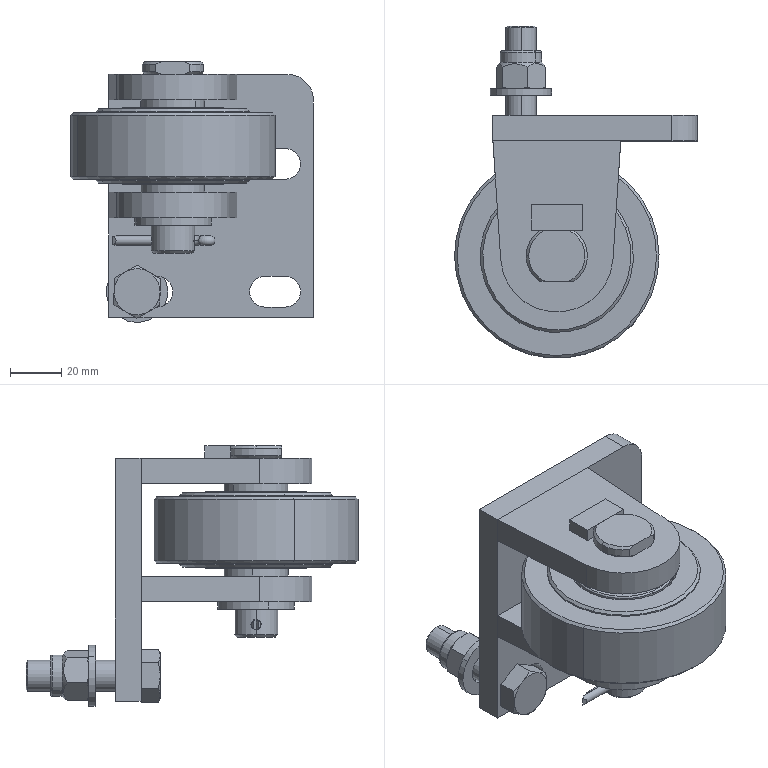Part | SolidWorks | features CompositeCurve 1 | 42 solids | 545 faces | box 95 x 130 x 102 mm | volume 277314 mm3 | cylinder 199 | plane 138 | sphere 104 | cone 52 | torus 52 | commonest cylinder face diameters 27.35 x46 29.65 x46 17 x14 60 x12 12 x8 24.667 x8